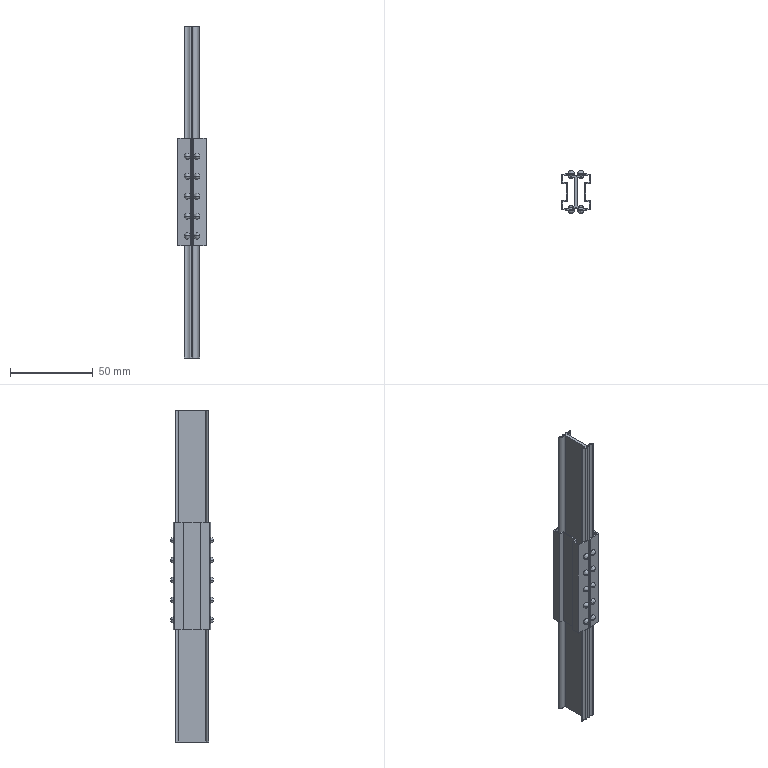Part | SolidWorks | features BaseBody 3 | 3 solids | 134 faces | box 17.1 x 26 x 200 mm | volume 15191 mm3 | spline 70 | plane 48 | cylinder 16 | commonest cylinder face diameters 3.7 x8 1 x4 2 x4